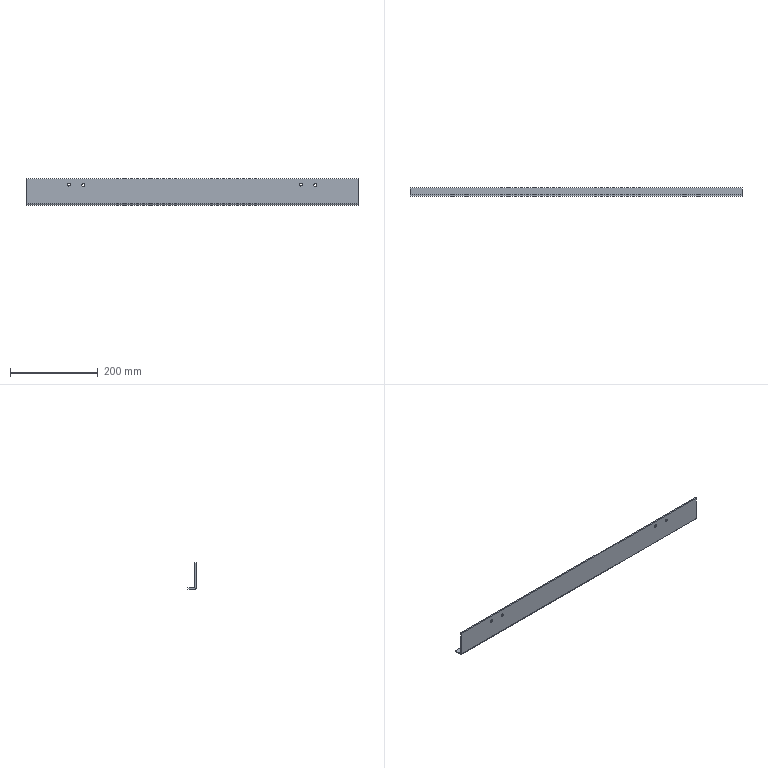Part | STEP file | HESS-408-70-15W-W-46-outer case reinforcing rib 5 | 1 solid | 18 faces | box 755 x 18.5 x 60 mm | volume 169016 mm3 | cylinder 10 | plane 8 | commonest cylinder face diameters 6.8 x8 0.2 x1 6.2 x1
STEP:
#1=CARTESIAN_POINT('',(0.,0.,0.));
#2=DIRECTION('',(0.,0.,1.));
#3=DIRECTION('',(1.,0.,0.));
#4=AXIS2_PLACEMENT_3D('',#1,#2,#3);
#5=CARTESIAN_POINT('',(-247.,0.,12.1));
#6=VERTEX_POINT('',#5);
#7=CARTESIAN_POINT('',(-247.,-3.,12.1));
#8=VERTEX_POINT('',#7);
#9=CARTESIAN_POINT('',(-247.,7.,12.1));
#10=DIRECTION('',(0.,-1.,0.));
#11=VECTOR('',#10,1.);
#12=LINE('',#9,#11);
#13=CARTESIAN_POINT('',(-247.,7.,15.5));
#14=DIRECTION('',(0.,-1.,0.));
#15=DIRECTION('',(0.,0.,-1.));
#16=AXIS2_PLACEMENT_3D('',#13,#14,#15);
#17=CYLINDRICAL_SURFACE('',#16,3.4);
#18=CARTESIAN_POINT('',(6.283,0.));
#19=DIRECTION('',(0.,1.));
#20=VECTOR('',#19,1.);
#21=LINE('',#18,#20);
#22=(GEOMETRIC_REPRESENTATION_CONTEXT(2)PARAMETRIC_REPRESENTATION_CONTEXT()REPRESENTATION_CONTEXT('',''));
#23=DEFINITIONAL_REPRESENTATION('',(#21),#22);
#24=PCURVE('',#17,#23);
#25=CARTESIAN_POINT('',(-247.,7.,15.5));
#26=DIRECTION('',(0.,-1.,0.));
#27=DIRECTION('',(0.,0.,-1.));
#28=AXIS2_PLACEMENT_3D('',#25,#26,#27);
#29=CYLINDRICAL_SURFACE('',#28,3.4);
#30=CARTESIAN_POINT('',(0.,0.));
#31=DIRECTION('',(0.,1.));
#32=VECTOR('',#31,1.);
#33=LINE('',#30,#32);
#34=(GEOMETRIC_REPRESENTATION_CONTEXT(2)PARAMETRIC_REPRESENTATION_CONTEXT()REPRESENTATION_CONTEXT('',''));
#35=DEFINITIONAL_REPRESENTATION('',(#33),#34);
#36=PCURVE('',#29,#35);
#37=SURFACE_CURVE('',#12,(#24,#36),.PCURVE_S1.);
#38=EDGE_CURVE('',#6,#8,#37,.T.);
#39=ORIENTED_EDGE('',*,*,#38,.T.);
#40=CARTESIAN_POINT('',(-247.,-3.,18.9));
#41=VERTEX_POINT('',#40);
#42=CARTESIAN_POINT('',(-247.,-3.,15.5));
#43=DIRECTION('',(0.,1.,0.));
#44=DIRECTION('',(0.,0.,-1.));
#45=AXIS2_PLACEMENT_3D('',#42,#43,#44);
#46=CIRCLE('',#45,3.4);
#47=CARTESIAN_POINT('',(6.283,10.));
#48=DIRECTION('',(-1.,0.));
#49=VECTOR('',#48,1.);
#50=LINE('',#47,#49);
#51=(GEOMETRIC_REPRESENTATION_CONTEXT(2)PARAMETRIC_REPRESENTATION_CONTEXT()REPRESENTATION_CONTEXT('',''));
#52=DEFINITIONAL_REPRESENTATION('',(#50),#51);
#53=PCURVE('',#17,#52);
#54=CARTESIAN_POINT('',(0.,-3.,0.));
#55=DIRECTION('',(0.,-1.,0.));
#56=DIRECTION('',(0.,0.,-1.));
#57=AXIS2_PLACEMENT_3D('',#54,#55,#56);
#58=PLANE('',#57);
#59=CARTESIAN_POINT('',(-12.1,-247.));
#60=CARTESIAN_POINT('',(-12.1,-252.889));
#61=CARTESIAN_POINT('',(-17.2,-249.944));
#62=CARTESIAN_POINT('',(-22.3,-247.));
#63=CARTESIAN_POINT('',(-17.2,-244.056));
#64=CARTESIAN_POINT('',(-12.1,-241.111));
#65=CARTESIAN_POINT('',(-12.1,-247.));
#66=(BOUNDED_CURVE()B_SPLINE_CURVE(2,(#59,#60,#61,#62,#63,#64,#65),.UNSPECIFIED.,.T.,.F.)B_SPLINE_CURVE_WITH_KNOTS((1,2,2,2,2,1),(-2.094,0.,2.094,4.189,6.283,8.378),.UNSPECIFIED.)CURVE()GEOMETRIC_REPRESENTATION_ITEM()RATIONAL_B_SPLINE_CURVE((1.,0.5,1.,0.5,1.,0.5,1.))REPRESENTATION_ITEM(''));
#67=(GEOMETRIC_REPRESENTATION_CONTEXT(2)PARAMETRIC_REPRESENTATION_CONTEXT()REPRESENTATION_CONTEXT('',''));
#68=DEFINITIONAL_REPRESENTATION('',(#66),#67);
#69=PCURVE('',#58,#68);
#70=SURFACE_CURVE('',#46,(#53,#69),.PCURVE_S1.);
#71=EDGE_CURVE('',#8,#41,#70,.T.);
#72=ORIENTED_EDGE('',*,*,#71,.T.);
#73=CARTESIAN_POINT('',(-247.,0.,18.9));
#74=VERTEX_POINT('',#73);
#75=CARTESIAN_POINT('',(-247.,7.,18.9));
#76=DIRECTION('',(0.,-1.,0.));
#77=VECTOR('',#76,1.);
#78=LINE('',#75,#77);
#79=CARTESIAN_POINT('',(3.142,0.));
#80=DIRECTION('',(0.,1.));
#81=VECTOR('',#80,1.);
#82=LINE('',#79,#81);
#83=(GEOMETRIC_REPRESENTATION_CONTEXT(2)PARAMETRIC_REPRESENTATION_CONTEXT()REPRESENTATION_CONTEXT('',''));
#84=DEFINITIONAL_REPRESENTATION('',(#82),#83);
#85=PCURVE('',#17,#84);
#86=CARTESIAN_POINT('',(3.142,0.));
#87=DIRECTION('',(0.,1.));
#88=VECTOR('',#87,1.);
#89=LINE('',#86,#88);
#90=(GEOMETRIC_REPRESENTATION_CONTEXT(2)PARAMETRIC_REPRESENTATION_CONTEXT()REPRESENTATION_CONTEXT('',''));
#91=DEFINITIONAL_REPRESENTATION('',(#89),#90);
#92=PCURVE('',#29,#91);
#93=SURFACE_CURVE('',#78,(#85,#92),.PCURVE_S1.);
#94=EDGE_CURVE('',#74,#41,#93,.T.);
#95=ORIENTED_EDGE('',*,*,#94,.F.);
#96=CARTESIAN_POINT('',(-247.,0.,15.5));
#97=DIRECTION('',(0.,-1.,0.));
#98=DIRECTION('',(0.,0.,-1.));
#99=AXIS2_PLACEMENT_3D('',#96,#97,#98);
#100=CIRCLE('',#99,3.4);
#101=CARTESIAN_POINT('',(0.,7.));
#102=DIRECTION('',(1.,0.));
#103=VECTOR('',#102,1.);
#104=LINE('',#101,#103);
#105=(GEOMETRIC_REPRESENTATION_CONTEXT(2)PARAMETRIC_REPRESENTATION_CONTEXT()REPRESENTATION_CONTEXT('',''));
#106=DEFINITIONAL_REPRESENTATION('',(#104),#105);
#107=PCURVE('',#17,#106);
#108=CARTESIAN_POINT('',(0.,0.,0.));
#109=DIRECTION('',(0.,-1.,0.));
#110=DIRECTION('',(0.,0.,-1.));
#111=AXIS2_PLACEMENT_3D('',#108,#109,#110);
#112=PLANE('',#111);
#113=CARTESIAN_POINT('',(-15.5,-247.));
#114=DIRECTION('',(1.,0.));
#115=AXIS2_PLACEMENT_2D('',#113,#114);
#116=CIRCLE('',#115,3.4);
#117=(GEOMETRIC_REPRESENTATION_CONTEXT(2)PARAMETRIC_REPRESENTATION_CONTEXT()REPRESENTATION_CONTEXT('',''));
#118=DEFINITIONAL_REPRESENTATION('',(#116),#117);
#119=PCURVE('',#112,#118);
#120=SURFACE_CURVE('',#100,(#107,#119),.PCURVE_S1.);
#121=EDGE_CURVE('',#74,#6,#120,.T.);
#122=ORIENTED_EDGE('',*,*,#121,.T.);
#123=EDGE_LOOP('',(#39,#72,#95,#122));
#124=FACE_BOUND('',#123,.F.);
#125=ADVANCED_FACE('',(#124),#17,.F.);
#126=CARTESIAN_POINT('',(280.5,0.,12.1));
#127=VERTEX_POINT('',#126);
#128=CARTESIAN_POINT('',(280.5,-3.,12.1));
#129=VERTEX_POINT('',#128);
#130=CARTESIAN_POINT('',(280.5,7.,12.1));
#131=DIRECTION('',(0.,-1.,0.));
#132=VECTOR('',#131,1.);
#133=LINE('',#130,#132);
#134=CARTESIAN_POINT('',(280.5,7.,15.5));
#135=DIRECTION('',(0.,-1.,0.));
#136=DIRECTION('',(0.,0.,-1.));
#137=AXIS2_PLACEMENT_3D('',#134,#135,#136);
#138=CYLINDRICAL_SURFACE('',#137,3.4);
#139=CARTESIAN_POINT('',(6.283,0.));
#140=DIRECTION('',(0.,1.));
#141=VECTOR('',#140,1.);
#142=LINE('',#139,#141);
#143=(GEOMETRIC_REPRESENTATION_CONTEXT(2)PARAMETRIC_REPRESENTATION_CONTEXT()REPRESENTATION_CONTEXT('',''));
#144=DEFINITIONAL_REPRESENTATION('',(#142),#143);
#145=PCURVE('',#138,#144);
#146=CARTESIAN_POINT('',(280.5,7.,15.5));
#147=DIRECTION('',(0.,-1.,0.));
#148=DIRECTION('',(0.,0.,-1.));
#149=AXIS2_PLACEMENT_3D('',#146,#147,#148);
#150=CYLINDRICAL_SURFACE('',#149,3.4);
#151=CARTESIAN_POINT('',(0.,0.));
#152=DIRECTION('',(0.,1.));
#153=VECTOR('',#152,1.);
#154=LINE('',#151,#153);
#155=(GEOMETRIC_REPRESENTATION_CONTEXT(2)PARAMETRIC_REPRESENTATION_CONTEXT()REPRESENTATION_CONTEXT('',''));
#156=DEFINITIONAL_REPRESENTATION('',(#154),#155);
#157=PCURVE('',#150,#156);
#158=SURFACE_CURVE('',#133,(#145,#157),.PCURVE_S1.);
#159=EDGE_CURVE('',#127,#129,#158,.T.);
#160=ORIENTED_EDGE('',*,*,#159,.T.);
#161=CARTESIAN_POINT('',(280.5,-3.,18.9));
#162=VERTEX_POINT('',#161);
#163=CARTESIAN_POINT('',(280.5,-3.,15.5));
#164=DIRECTION('',(0.,1.,0.));
#165=DIRECTION('',(0.,0.,-1.));
#166=AXIS2_PLACEMENT_3D('',#163,#164,#165);
#167=CIRCLE('',#166,3.4);
#168=CARTESIAN_POINT('',(6.283,10.));
#169=DIRECTION('',(-1.,0.));
#170=VECTOR('',#169,1.);
#171=LINE('',#168,#170);
#172=(GEOMETRIC_REPRESENTATION_CONTEXT(2)PARAMETRIC_REPRESENTATION_CONTEXT()REPRESENTATION_CONTEXT('',''));
#173=DEFINITIONAL_REPRESENTATION('',(#171),#172);
#174=PCURVE('',#138,#173);
#175=CARTESIAN_POINT('',(-12.1,280.5));
#176=CARTESIAN_POINT('',(-12.1,274.611));
#177=CARTESIAN_POINT('',(-17.2,277.556));
#178=CARTESIAN_POINT('',(-22.3,280.5));
#179=CARTESIAN_POINT('',(-17.2,283.444));
#180=CARTESIAN_POINT('',(-12.1,286.389));
#181=CARTESIAN_POINT('',(-12.1,280.5));
#182=(BOUNDED_CURVE()B_SPLINE_CURVE(2,(#175,#176,#177,#178,#179,#180,#181),.UNSPECIFIED.,.T.,.F.)B_SPLINE_CURVE_WITH_KNOTS((1,2,2,2,2,1),(-2.094,0.,2.094,4.189,6.283,8.378),.UNSPECIFIED.)CURVE()GEOMETRIC_REPRESENTATION_ITEM()RATIONAL_B_SPLINE_CURVE((1.,0.5,1.,0.5,1.,0.5,1.))REPRESENTATION_ITEM(''));
#183=(GEOMETRIC_REPRESENTATION_CONTEXT(2)PARAMETRIC_REPRESENTATION_CONTEXT()REPRESENTATION_CONTEXT('',''));
#184=DEFINITIONAL_REPRESENTATION('',(#182),#183);
#185=PCURVE('',#58,#184);
#186=SURFACE_CURVE('',#167,(#174,#185),.PCURVE_S1.);
#187=EDGE_CURVE('',#129,#162,#186,.T.);
#188=ORIENTED_EDGE('',*,*,#187,.T.);
#189=CARTESIAN_POINT('',(280.5,0.,18.9));
#190=VERTEX_POINT('',#189);
#191=CARTESIAN_POINT('',(280.5,7.,18.9));
#192=DIRECTION('',(0.,-1.,0.));
#193=VECTOR('',#192,1.);
#194=LINE('',#191,#193);
#195=CARTESIAN_POINT('',(3.142,0.));
#196=DIRECTION('',(0.,1.));
#197=VECTOR('',#196,1.);
#198=LINE('',#195,#197);
#199=(GEOMETRIC_REPRESENTATION_CONTEXT(2)PARAMETRIC_REPRESENTATION_CONTEXT()REPRESENTATION_CONTEXT('',''));
#200=DEFINITIONAL_REPRESENTATION('',(#198),#199);
#201=PCURVE('',#138,#200);
#202=CARTESIAN_POINT('',(3.142,0.));
#203=DIRECTION('',(0.,1.));
#204=VECTOR('',#203,1.);
#205=LINE('',#202,#204);
#206=(GEOMETRIC_REPRESENTATION_CONTEXT(2)PARAMETRIC_REPRESENTATION_CONTEXT()REPRESENTATION_CONTEXT('',''));
#207=DEFINITIONAL_REPRESENTATION('',(#205),#206);
#208=PCURVE('',#150,#207);
#209=SURFACE_CURVE('',#194,(#201,#208),.PCURVE_S1.);
#210=EDGE_CURVE('',#190,#162,#209,.T.);
#211=ORIENTED_EDGE('',*,*,#210,.F.);
#212=CARTESIAN_POINT('',(280.5,0.,15.5));
#213=DIRECTION('',(0.,-1.,0.));
#214=DIRECTION('',(0.,0.,-1.));
#215=AXIS2_PLACEMENT_3D('',#212,#213,#214);
#216=CIRCLE('',#215,3.4);
#217=CARTESIAN_POINT('',(0.,7.));
#218=DIRECTION('',(1.,0.));
#219=VECTOR('',#218,1.);
#220=LINE('',#217,#219);
#221=(GEOMETRIC_REPRESENTATION_CONTEXT(2)PARAMETRIC_REPRESENTATION_CONTEXT()REPRESENTATION_CONTEXT('',''));
#222=DEFINITIONAL_REPRESENTATION('',(#220),#221);
#223=PCURVE('',#138,#222);
#224=CARTESIAN_POINT('',(-15.5,280.5));
#225=DIRECTION('',(1.,0.));
#226=AXIS2_PLACEMENT_2D('',#224,#225);
#227=CIRCLE('',#226,3.4);
#228=(GEOMETRIC_REPRESENTATION_CONTEXT(2)PARAMETRIC_REPRESENTATION_CONTEXT()REPRESENTATION_CONTEXT('',''));
#229=DEFINITIONAL_REPRESENTATION('',(#227),#228);
#230=PCURVE('',#112,#229);
#231=SURFACE_CURVE('',#216,(#223,#230),.PCURVE_S1.);
#232=EDGE_CURVE('',#190,#127,#231,.T.);
#233=ORIENTED_EDGE('',*,*,#232,.T.);
#234=EDGE_LOOP('',(#160,#188,#211,#233));
#235=FACE_BOUND('',#234,.F.);
#236=ADVANCED_FACE('',(#235),#138,.F.);
#237=CARTESIAN_POINT('',(247.,0.,13.6));
#238=VERTEX_POINT('',#237);
#239=CARTESIAN_POINT('',(247.,-3.,13.6));
#240=VERTEX_POINT('',#239);
#241=CARTESIAN_POINT('',(247.,7.,13.6));
#242=DIRECTION('',(0.,-1.,0.));
#243=VECTOR('',#242,1.);
#244=LINE('',#241,#243);
#245=CARTESIAN_POINT('',(247.,7.,17.));
#246=DIRECTION('',(0.,-1.,0.));
#247=DIRECTION('',(0.,0.,-1.));
#248=AXIS2_PLACEMENT_3D('',#245,#246,#247);
#249=CYLINDRICAL_SURFACE('',#248,3.4);
#250=CARTESIAN_POINT('',(6.283,0.));
#251=DIRECTION('',(0.,1.));
#252=VECTOR('',#251,1.);
#253=LINE('',#250,#252);
#254=(GEOMETRIC_REPRESENTATION_CONTEXT(2)PARAMETRIC_REPRESENTATION_CONTEXT()REPRESENTATION_CONTEXT('',''));
#255=DEFINITIONAL_REPRESENTATION('',(#253),#254);
#256=PCURVE('',#249,#255);
#257=CARTESIAN_POINT('',(247.,7.,17.));
#258=DIRECTION('',(0.,-1.,0.));
#259=DIRECTION('',(0.,0.,-1.));
#260=AXIS2_PLACEMENT_3D('',#257,#258,#259);
#261=CYLINDRICAL_SURFACE('',#260,3.4);
#262=CARTESIAN_POINT('',(0.,0.));
#263=DIRECTION('',(0.,1.));
#264=VECTOR('',#263,1.);
#265=LINE('',#262,#264);
#266=(GEOMETRIC_REPRESENTATION_CONTEXT(2)PARAMETRIC_REPRESENTATION_CONTEXT()REPRESENTATION_CONTEXT('',''));
#267=DEFINITIONAL_REPRESENTATION('',(#265),#266);
#268=PCURVE('',#261,#267);
#269=SURFACE_CURVE('',#244,(#256,#268),.PCURVE_S1.);
#270=EDGE_CURVE('',#238,#240,#269,.T.);
#271=ORIENTED_EDGE('',*,*,#270,.T.);
#272=CARTESIAN_POINT('',(247.,-3.,20.4));
#273=VERTEX_POINT('',#272);
#274=CARTESIAN_POINT('',(247.,-3.,17.));
#275=DIRECTION('',(0.,1.,0.));
#276=DIRECTION('',(0.,0.,-1.));
#277=AXIS2_PLACEMENT_3D('',#274,#275,#276);
#278=CIRCLE('',#277,3.4);
#279=CARTESIAN_POINT('',(6.283,10.));
#280=DIRECTION('',(-1.,0.));
#281=VECTOR('',#280,1.);
#282=LINE('',#279,#281);
#283=(GEOMETRIC_REPRESENTATION_CONTEXT(2)PARAMETRIC_REPRESENTATION_CONTEXT()REPRESENTATION_CONTEXT('',''));
#284=DEFINITIONAL_REPRESENTATION('',(#282),#283);
#285=PCURVE('',#249,#284);
#286=CARTESIAN_POINT('',(-13.6,247.));
#287=CARTESIAN_POINT('',(-13.6,241.111));
#288=CARTESIAN_POINT('',(-18.7,244.056));
#289=CARTESIAN_POINT('',(-23.8,247.));
#290=CARTESIAN_POINT('',(-18.7,249.944));
#291=CARTESIAN_POINT('',(-13.6,252.889));
#292=CARTESIAN_POINT('',(-13.6,247.));
#293=(BOUNDED_CURVE()B_SPLINE_CURVE(2,(#286,#287,#288,#289,#290,#291,#292),.UNSPECIFIED.,.T.,.F.)B_SPLINE_CURVE_WITH_KNOTS((1,2,2,2,2,1),(-2.094,0.,2.094,4.189,6.283,8.378),.UNSPECIFIED.)CURVE()GEOMETRIC_REPRESENTATION_ITEM()RATIONAL_B_SPLINE_CURVE((1.,0.5,1.,0.5,1.,0.5,1.))REPRESENTATION_ITEM(''));
#294=(GEOMETRIC_REPRESENTATION_CONTEXT(2)PARAMETRIC_REPRESENTATION_CONTEXT()REPRESENTATION_CONTEXT('',''));
#295=DEFINITIONAL_REPRESENTATION('',(#293),#294);
#296=PCURVE('',#58,#295);
#297=SURFACE_CURVE('',#278,(#285,#296),.PCURVE_S1.);
#298=EDGE_CURVE('',#240,#273,#297,.T.);
#299=ORIENTED_EDGE('',*,*,#298,.T.);
#300=CARTESIAN_POINT('',(247.,0.,20.4));
#301=VERTEX_POINT('',#300);
#302=CARTESIAN_POINT('',(247.,7.,20.4));
#303=DIRECTION('',(0.,-1.,0.));
#304=VECTOR('',#303,1.);
#305=LINE('',#302,#304);
#306=CARTESIAN_POINT('',(3.142,0.));
#307=DIRECTION('',(0.,1.));
#308=VECTOR('',#307,1.);
#309=LINE('',#306,#308);
#310=(GEOMETRIC_REPRESENTATION_CONTEXT(2)PARAMETRIC_REPRESENTATION_CONTEXT()REPRESENTATION_CONTEXT('',''));
#311=DEFINITIONAL_REPRESENTATION('',(#309),#310);
#312=PCURVE('',#249,#311);
#313=CARTESIAN_POINT('',(3.142,0.));
#314=DIRECTION('',(0.,1.));
#315=VECTOR('',#314,1.);
#316=LINE('',#313,#315);
#317=(GEOMETRIC_REPRESENTATION_CONTEXT(2)PARAMETRIC_REPRESENTATION_CONTEXT()REPRESENTATION_CONTEXT('',''));
#318=DEFINITIONAL_REPRESENTATION('',(#316),#317);
#319=PCURVE('',#261,#318);
#320=SURFACE_CURVE('',#305,(#312,#319),.PCURVE_S1.);
#321=EDGE_CURVE('',#301,#273,#320,.T.);
#322=ORIENTED_EDGE('',*,*,#321,.F.);
#323=CARTESIAN_POINT('',(247.,0.,17.));
#324=DIRECTION('',(0.,-1.,0.));
#325=DIRECTION('',(0.,0.,-1.));
#326=AXIS2_PLACEMENT_3D('',#323,#324,#325);
#327=CIRCLE('',#326,3.4);
#328=CARTESIAN_POINT('',(0.,7.));
#329=DIRECTION('',(1.,0.));
#330=VECTOR('',#329,1.);
#331=LINE('',#328,#330);
#332=(GEOMETRIC_REPRESENTATION_CONTEXT(2)PARAMETRIC_REPRESENTATION_CONTEXT()REPRESENTATION_CONTEXT('',''));
#333=DEFINITIONAL_REPRESENTATION('',(#331),#332);
#334=PCURVE('',#249,#333);
#335=CARTESIAN_POINT('',(-17.,247.));
#336=DIRECTION('',(1.,0.));
#337=AXIS2_PLACEMENT_2D('',#335,#336);
#338=CIRCLE('',#337,3.4);
#339=(GEOMETRIC_REPRESENTATION_CONTEXT(2)PARAMETRIC_REPRESENTATION_CONTEXT()REPRESENTATION_CONTEXT('',''));
#340=DEFINITIONAL_REPRESENTATION('',(#338),#339);
#341=PCURVE('',#112,#340);
#342=SURFACE_CURVE('',#327,(#334,#341),.PCURVE_S1.);
#343=EDGE_CURVE('',#301,#238,#342,.T.);
#344=ORIENTED_EDGE('',*,*,#343,.T.);
#345=EDGE_LOOP('',(#271,#299,#322,#344));
#346=FACE_BOUND('',#345,.F.);
#347=ADVANCED_FACE('',(#346),#249,.F.);
#348=CARTESIAN_POINT('',(-280.5,0.,13.6));
#349=VERTEX_POINT('',#348);
#350=CARTESIAN_POINT('',(-280.5,-3.,13.6));
#351=VERTEX_POINT('',#350);
#352=CARTESIAN_POINT('',(-280.5,7.,13.6));
#353=DIRECTION('',(0.,-1.,0.));
#354=VECTOR('',#353,1.);
#355=LINE('',#352,#354);
#356=CARTESIAN_POINT('',(-280.5,7.,17.));
#357=DIRECTION('',(0.,-1.,0.));
#358=DIRECTION('',(0.,0.,-1.));
#359=AXIS2_PLACEMENT_3D('',#356,#357,#358);
#360=CYLINDRICAL_SURFACE('',#359,3.4);
#361=CARTESIAN_POINT('',(6.283,0.));
#362=DIRECTION('',(0.,1.));
#363=VECTOR('',#362,1.);
#364=LINE('',#361,#363);
#365=(GEOMETRIC_REPRESENTATION_CONTEXT(2)PARAMETRIC_REPRESENTATION_CONTEXT()REPRESENTATION_CONTEXT('',''));
#366=DEFINITIONAL_REPRESENTATION('',(#364),#365);
#367=PCURVE('',#360,#366);
#368=CARTESIAN_POINT('',(-280.5,7.,17.));
#369=DIRECTION('',(0.,-1.,0.));
#370=DIRECTION('',(0.,0.,-1.));
#371=AXIS2_PLACEMENT_3D('',#368,#369,#370);
#372=CYLINDRICAL_SURFACE('',#371,3.4);
#373=CARTESIAN_POINT('',(0.,0.));
#374=DIRECTION('',(0.,1.));
#375=VECTOR('',#374,1.);
#376=LINE('',#373,#375);
#377=(GEOMETRIC_REPRESENTATION_CONTEXT(2)PARAMETRIC_REPRESENTATION_CONTEXT()REPRESENTATION_CONTEXT('',''));
#378=DEFINITIONAL_REPRESENTATION('',(#376),#377);
#379=PCURVE('',#372,#378);
#380=SURFACE_CURVE('',#355,(#367,#379),.PCURVE_S1.);
#381=EDGE_CURVE('',#349,#351,#380,.T.);
#382=ORIENTED_EDGE('',*,*,#381,.T.);
#383=CARTESIAN_POINT('',(-280.5,-3.,20.4));
#384=VERTEX_POINT('',#383);
#385=CARTESIAN_POINT('',(-280.5,-3.,17.));
#386=DIRECTION('',(0.,1.,0.));
#387=DIRECTION('',(0.,0.,-1.));
#388=AXIS2_PLACEMENT_3D('',#385,#386,#387);
#389=CIRCLE('',#388,3.4);
#390=CARTESIAN_POINT('',(6.283,10.));
#391=DIRECTION('',(-1.,0.));
#392=VECTOR('',#391,1.);
#393=LINE('',#390,#392);
#394=(GEOMETRIC_REPRESENTATION_CONTEXT(2)PARAMETRIC_REPRESENTATION_CONTEXT()REPRESENTATION_CONTEXT('',''));
#395=DEFINITIONAL_REPRESENTATION('',(#393),#394);
#396=PCURVE('',#360,#395);
#397=CARTESIAN_POINT('',(-13.6,-280.5));
#398=CARTESIAN_POINT('',(-13.6,-286.389));
#399=CARTESIAN_POINT('',(-18.7,-283.444));
#400=CARTESIAN_POINT('',(-23.8,-280.5));
#401=CARTESIAN_POINT('',(-18.7,-277.556));
#402=CARTESIAN_POINT('',(-13.6,-274.611));
#403=CARTESIAN_POINT('',(-13.6,-280.5));
#404=(BOUNDED_CURVE()B_SPLINE_CURVE(2,(#397,#398,#399,#400,#401,#402,#403),.UNSPECIFIED.,.T.,.F.)B_SPLINE_CURVE_WITH_KNOTS((1,2,2,2,2,1),(-2.094,0.,2.094,4.189,6.283,8.378),.UNSPECIFIED.)CURVE()GEOMETRIC_REPRESENTATION_ITEM()RATIONAL_B_SPLINE_CURVE((1.,0.5,1.,0.5,1.,0.5,1.))REPRESENTATION_ITEM(''));
#405=(GEOMETRIC_REPRESENTATION_CONTEXT(2)PARAMETRIC_REPRESENTATION_CONTEXT()REPRESENTATION_CONTEXT('',''));
#406=DEFINITIONAL_REPRESENTATION('',(#404),#405);
#407=PCURVE('',#58,#406);
#408=SURFACE_CURVE('',#389,(#396,#407),.PCURVE_S1.);
#409=EDGE_CURVE('',#351,#384,#408,.T.);
#410=ORIENTED_EDGE('',*,*,#409,.T.);
#411=CARTESIAN_POINT('',(-280.5,0.,20.4));
#412=VERTEX_POINT('',#411);
#413=CARTESIAN_POINT('',(-280.5,7.,20.4));
#414=DIRECTION('',(0.,-1.,0.));
#415=VECTOR('',#414,1.);
#416=LINE('',#413,#415);
#417=CARTESIAN_POINT('',(3.142,0.));
#418=DIRECTION('',(0.,1.));
#419=VECTOR('',#418,1.);
#420=LINE('',#417,#419);
#421=(GEOMETRIC_REPRESENTATION_CONTEXT(2)PARAMETRIC_REPRESENTATION_CONTEXT()REPRESENTATION_CONTEXT('',''));
#422=DEFINITIONAL_REPRESENTATION('',(#420),#421);
#423=PCURVE('',#360,#422);
#424=CARTESIAN_POINT('',(3.142,0.));
#425=DIRECTION('',(0.,1.));
#426=VECTOR('',#425,1.);
#427=LINE('',#424,#426);
#428=(GEOMETRIC_REPRESENTATION_CONTEXT(2)PARAMETRIC_REPRESENTATION_CONTEXT()REPRESENTATION_CONTEXT('',''));
#429=DEFINITIONAL_REPRESENTATION('',(#427),#428);
#430=PCURVE('',#372,#429);
#431=SURFACE_CURVE('',#416,(#423,#430),.PCURVE_S1.);
#432=EDGE_CURVE('',#412,#384,#431,.T.);
#433=ORIENTED_EDGE('',*,*,#432,.F.);
#434=CARTESIAN_POINT('',(-280.5,0.,17.));
#435=DIRECTION('',(0.,-1.,0.));
#436=DIRECTION('',(0.,0.,-1.));
#437=AXIS2_PLACEMENT_3D('',#434,#435,#436);
#438=CIRCLE('',#437,3.4);
#439=CARTESIAN_POINT('',(0.,7.));
#440=DIRECTION('',(1.,0.));
#441=VECTOR('',#440,1.);
#442=LINE('',#439,#441);
#443=(GEOMETRIC_REPRESENTATION_CONTEXT(2)PARAMETRIC_REPRESENTATION_CONTEXT()REPRESENTATION_CONTEXT('',''));
#444=DEFINITIONAL_REPRESENTATION('',(#442),#443);
#445=PCURVE('',#360,#444);
#446=CARTESIAN_POINT('',(-17.,-280.5));
#447=DIRECTION('',(1.,0.));
#448=AXIS2_PLACEMENT_2D('',#446,#447);
#449=CIRCLE('',#448,3.4);
#450=(GEOMETRIC_REPRESENTATION_CONTEXT(2)PARAMETRIC_REPRESENTATION_CONTEXT()REPRESENTATION_CONTEXT('',''));
#451=DEFINITIONAL_REPRESENTATION('',(#449),#450);
#452=PCURVE('',#112,#451);
#453=SURFACE_CURVE('',#438,(#445,#452),.PCURVE_S1.);
#454=EDGE_CURVE('',#412,#349,#453,.T.);
#455=ORIENTED_EDGE('',*,*,#454,.T.);
#456=EDGE_LOOP('',(#382,#410,#433,#455));
#457=FACE_BOUND('',#456,.F.);
#458=ADVANCED_FACE('',(#457),#360,.F.);
#459=CARTESIAN_POINT('',(377.5,-3.,-26.9));
#460=VERTEX_POINT('',#459);
#461=CARTESIAN_POINT('',(377.5,-3.,30.));
#462=VERTEX_POINT('',#461);
#463=CARTESIAN_POINT('',(377.5,-3.,0.));
#464=DIRECTION('',(0.,0.,1.));
#465=VECTOR('',#464,1.);
#466=LINE('',#463,#465);
#467=CARTESIAN_POINT('',(0.,377.5));
#468=DIRECTION('',(-1.,0.));
#469=VECTOR('',#468,1.);
#470=LINE('',#467,#469);
#471=(GEOMETRIC_REPRESENTATION_CONTEXT(2)PARAMETRIC_REPRESENTATION_CONTEXT()REPRESENTATION_CONTEXT('',''));
#472=DEFINITIONAL_REPRESENTATION('',(#470),#471);
#473=PCURVE('',#58,#472);
#474=CARTESIAN_POINT('',(377.5,-3.,30.));
#475=DIRECTION('',(1.,0.,0.));
#476=DIRECTION('',(0.,0.,-1.));
#477=AXIS2_PLACEMENT_3D('',#474,#475,#476);
#478=PLANE('',#477);
#479=CARTESIAN_POINT('',(30.,0.));
#480=DIRECTION('',(-1.,0.));
#481=VECTOR('',#480,1.);
#482=LINE('',#479,#481);
#483=(GEOMETRIC_REPRESENTATION_CONTEXT(2)PARAMETRIC_REPRESENTATION_CONTEXT()REPRESENTATION_CONTEXT('',''));
#484=DEFINITIONAL_REPRESENTATION('',(#482),#483);
#485=PCURVE('',#478,#484);
#486=SURFACE_CURVE('',#466,(#473,#485),.PCURVE_S1.);
#487=EDGE_CURVE('',#460,#462,#486,.T.);
#488=ORIENTED_EDGE('',*,*,#487,.T.);
#489=CARTESIAN_POINT('',(-377.5,-3.,30.));
#490=VERTEX_POINT('',#489);
#491=CARTESIAN_POINT('',(0.,-3.,30.));
#492=DIRECTION('',(-1.,0.,0.));
#493=VECTOR('',#492,1.);
#494=LINE('',#491,#493);
#495=CARTESIAN_POINT('',(-30.,0.));
#496=DIRECTION('',(0.,-1.));
#497=VECTOR('',#496,1.);
#498=LINE('',#495,#497);
#499=(GEOMETRIC_REPRESENTATION_CONTEXT(2)PARAMETRIC_REPRESENTATION_CONTEXT()REPRESENTATION_CONTEXT('',''));
#500=DEFINITIONAL_REPRESENTATION('',(#498),#499);
#501=PCURVE('',#58,#500);
#502=CARTESIAN_POINT('',(-377.5,-3.,30.));
#503=DIRECTION('',(0.,0.,1.));
#504=DIRECTION('',(1.,0.,0.));
#505=AXIS2_PLACEMENT_3D('',#502,#503,#504);
#506=PLANE('',#505);
#507=CARTESIAN_POINT('',(377.5,0.));
#508=DIRECTION('',(-1.,0.));
#509=VECTOR('',#508,1.);
#510=LINE('',#507,#509);
#511=(GEOMETRIC_REPRESENTATION_CONTEXT(2)PARAMETRIC_REPRESENTATION_CONTEXT()REPRESENTATION_CONTEXT('',''));
#512=DEFINITIONAL_REPRESENTATION('',(#510),#511);
#513=PCURVE('',#506,#512);
#514=SURFACE_CURVE('',#494,(#501,#513),.PCURVE_S1.);
#515=EDGE_CURVE('',#462,#490,#514,.T.);
#516=ORIENTED_EDGE('',*,*,#515,.T.);
#517=CARTESIAN_POINT('',(-377.5,-3.,-26.9));
#518=VERTEX_POINT('',#517);
#519=CARTESIAN_POINT('',(-377.5,-3.,0.));
#520=DIRECTION('',(0.,0.,-1.));
#521=VECTOR('',#520,1.);
#522=LINE('',#519,#521);
#523=CARTESIAN_POINT('',(0.,-377.5));
#524=DIRECTION('',(1.,0.));
#525=VECTOR('',#524,1.);
#526=LINE('',#523,#525);
#527=(GEOMETRIC_REPRESENTATION_CONTEXT(2)PARAMETRIC_REPRESENTATION_CONTEXT()REPRESENTATION_CONTEXT('',''));
#528=DEFINITIONAL_REPRESENTATION('',(#526),#527);
#529=PCURVE('',#58,#528);
#530=CARTESIAN_POINT('',(-377.5,-3.,30.));
#531=DIRECTION('',(-1.,0.,0.));
#532=DIRECTION('',(0.,0.,1.));
#533=AXIS2_PLACEMENT_3D('',#530,#531,#532);
#534=PLANE('',#533);
#535=CARTESIAN_POINT('',(-30.,0.));
#536=DIRECTION('',(-1.,0.));
#537=VECTOR('',#536,1.);
#538=LINE('',#535,#537);
#539=(GEOMETRIC_REPRESENTATION_CONTEXT(2)PARAMETRIC_REPRESENTATION_CONTEXT()REPRESENTATION_CONTEXT('',''));
#540=DEFINITIONAL_REPRESENTATION('',(#538),#539);
#541=PCURVE('',#534,#540);
#542=SURFACE_CURVE('',#522,(#529,#541),.PCURVE_S1.);
#543=EDGE_CURVE('',#490,#518,#542,.T.);
#544=ORIENTED_EDGE('',*,*,#543,.T.);
#545=CARTESIAN_POINT('',(0.,-3.,-26.9));
#546=DIRECTION('',(1.,0.,0.));
#547=VECTOR('',#546,1.);
#548=LINE('',#545,#547);
#549=CARTESIAN_POINT('',(26.9,0.));
#550=DIRECTION('',(0.,1.));
#551=VECTOR('',#550,1.);
#552=LINE('',#549,#551);
#553=(GEOMETRIC_REPRESENTATION_CONTEXT(2)PARAMETRIC_REPRESENTATION_CONTEXT()REPRESENTATION_CONTEXT('',''));
#554=DEFINITIONAL_REPRESENTATION('',(#552),#553);
#555=PCURVE('',#58,#554);
#556=CARTESIAN_POINT('',(-377.5,0.1,-26.9));
#557=DIRECTION('',(-1.,0.,0.));
#558=DIRECTION('',(0.,-1.,0.));
#559=AXIS2_PLACEMENT_3D('',#556,#557,#558);
#560=CYLINDRICAL_SURFACE('',#559,3.1);
#561=CARTESIAN_POINT('',(6.283,-377.5));
#562=DIRECTION('',(0.,-1.));
#563=VECTOR('',#562,1.);
#564=LINE('',#561,#563);
#565=(GEOMETRIC_REPRESENTATION_CONTEXT(2)PARAMETRIC_REPRESENTATION_CONTEXT()REPRESENTATION_CONTEXT('',''));
#566=DEFINITIONAL_REPRESENTATION('',(#564),#565);
#567=PCURVE('',#560,#566);
#568=SURFACE_CURVE('',#548,(#555,#567),.PCURVE_S1.);
#569=EDGE_CURVE('',#518,#460,#568,.T.);
#570=ORIENTED_EDGE('',*,*,#569,.T.);
#571=EDGE_LOOP('',(#488,#516,#544,#570));
#572=FACE_BOUND('',#571,.T.);
#573=ORIENTED_EDGE('',*,*,#71,.T.);
#574=CARTESIAN_POINT('',(-247.,-3.,15.5));
#575=DIRECTION('',(0.,1.,0.));
#576=DIRECTION('',(0.,0.,-1.));
#577=AXIS2_PLACEMENT_3D('',#574,#575,#576);
#578=CIRCLE('',#577,3.4);
#579=CARTESIAN_POINT('',(-12.1,-247.));
#580=CARTESIAN_POINT('',(-12.1,-252.889));
#581=CARTESIAN_POINT('',(-17.2,-249.944));
#582=CARTESIAN_POINT('',(-22.3,-247.));
#583=CARTESIAN_POINT('',(-17.2,-244.056));
#584=CARTESIAN_POINT('',(-12.1,-241.111));
#585=CARTESIAN_POINT('',(-12.1,-247.));
#586=(BOUNDED_CURVE()B_SPLINE_CURVE(2,(#579,#580,#581,#582,#583,#584,#585),.UNSPECIFIED.,.T.,.F.)B_SPLINE_CURVE_WITH_KNOTS((1,2,2,2,2,1),(-2.094,0.,2.094,4.189,6.283,8.378),.UNSPECIFIED.)CURVE()GEOMETRIC_REPRESENTATION_ITEM()RATIONAL_B_SPLINE_CURVE((1.,0.5,1.,0.5,1.,0.5,1.))REPRESENTATION_ITEM(''));
#587=(GEOMETRIC_REPRESENTATION_CONTEXT(2)PARAMETRIC_REPRESENTATION_CONTEXT()REPRESENTATION_CONTEXT('',''));
#588=DEFINITIONAL_REPRESENTATION('',(#586),#587);
#589=PCURVE('',#58,#588);
#590=CARTESIAN_POINT('',(6.283,10.));
#591=DIRECTION('',(-1.,0.));
#592=VECTOR('',#591,1.);
#593=LINE('',#590,#592);
#594=(GEOMETRIC_REPRESENTATION_CONTEXT(2)PARAMETRIC_REPRESENTATION_CONTEXT()REPRESENTATION_CONTEXT('',''));
#595=DEFINITIONAL_REPRESENTATION('',(#593),#594);
#596=PCURVE('',#29,#595);
#597=SURFACE_CURVE('',#578,(#589,#596),.PCURVE_S1.);
#598=EDGE_CURVE('',#41,#8,#597,.T.);
#599=ORIENTED_EDGE('',*,*,#598,.T.);
#600=EDGE_LOOP('',(#573,#599));
#601=FACE_BOUND('',#600,.T.);
#602=ORIENTED_EDGE('',*,*,#187,.T.);
#603=CARTESIAN_POINT('',(280.5,-3.,15.5));
#604=DIRECTION('',(0.,1.,0.));
#605=DIRECTION('',(0.,0.,-1.));
#606=AXIS2_PLACEMENT_3D('',#603,#604,#605);
#607=CIRCLE('',#606,3.4);
#608=CARTESIAN_POINT('',(-12.1,280.5));
#609=CARTESIAN_POINT('',(-12.1,274.611));
#610=CARTESIAN_POINT('',(-17.2,277.556));
#611=CARTESIAN_POINT('',(-22.3,280.5));
#612=CARTESIAN_POINT('',(-17.2,283.444));
#613=CARTESIAN_POINT('',(-12.1,286.389));
#614=CARTESIAN_POINT('',(-12.1,280.5));
#615=(BOUNDED_CURVE()B_SPLINE_CURVE(2,(#608,#609,#610,#611,#612,#613,#614),.UNSPECIFIED.,.T.,.F.)B_SPLINE_CURVE_WITH_KNOTS((1,2,2,2,2,1),(-2.094,0.,2.094,4.189,6.283,8.378),.UNSPECIFIED.)CURVE()GEOMETRIC_REPRESENTATION_ITEM()RATIONAL_B_SPLINE_CURVE((1.,0.5,1.,0.5,1.,0.5,1.))REPRESENTATION_ITEM(''));
#616=(GEOMETRIC_REPRESENTATION_CONTEXT(2)PARAMETRIC_REPRESENTATION_CONTEXT()REPRESENTATION_CONTEXT('',''));
#617=DEFINITIONAL_REPRESENTATION('',(#615),#616);
#618=PCURVE('',#58,#617);
#619=CARTESIAN_POINT('',(6.283,10.));
#620=DIRECTION('',(-1.,0.));
#621=VECTOR('',#620,1.);
#622=LINE('',#619,#621);
#623=(GEOMETRIC_REPRESENTATION_CONTEXT(2)PARAMETRIC_REPRESENTATION_CONTEXT()REPRESENTATION_CONTEXT('',''));
#624=DEFINITIONAL_REPRESENTATION('',(#622),#623);
#625=PCURVE('',#150,#624);
#626=SURFACE_CURVE('',#607,(#618,#625),.PCURVE_S1.);
#627=EDGE_CURVE('',#162,#129,#626,.T.);
#628=ORIENTED_EDGE('',*,*,#627,.T.);
#629=EDGE_LOOP('',(#602,#628));
#630=FACE_BOUND('',#629,.T.);
#631=ORIENTED_EDGE('',*,*,#298,.T.);
#632=CARTESIAN_POINT('',(247.,-3.,17.));
#633=DIRECTION('',(0.,1.,0.));
#634=DIRECTION('',(0.,0.,-1.));
#635=AXIS2_PLACEMENT_3D('',#632,#633,#634);
#636=CIRCLE('',#635,3.4);
#637=CARTESIAN_POINT('',(-13.6,247.));
#638=CARTESIAN_POINT('',(-13.6,241.111));
#639=CARTESIAN_POINT('',(-18.7,244.056));
#640=CARTESIAN_POINT('',(-23.8,247.));
#641=CARTESIAN_POINT('',(-18.7,249.944));
#642=CARTESIAN_POINT('',(-13.6,252.889));
#643=CARTESIAN_POINT('',(-13.6,247.));
#644=(BOUNDED_CURVE()B_SPLINE_CURVE(2,(#637,#638,#639,#640,#641,#642,#643),.UNSPECIFIED.,.T.,.F.)B_SPLINE_CURVE_WITH_KNOTS((1,2,2,2,2,1),(-2.094,0.,2.094,4.189,6.283,8.378),.UNSPECIFIED.)CURVE()GEOMETRIC_REPRESENTATION_ITEM()RATIONAL_B_SPLINE_CURVE((1.,0.5,1.,0.5,1.,0.5,1.))REPRESENTATION_ITEM(''));
#645=(GEOMETRIC_REPRESENTATION_CONTEXT(2)PARAMETRIC_REPRESENTATION_CONTEXT()REPRESENTATION_CONTEXT('',''));
#646=DEFINITIONAL_REPRESENTATION('',(#644),#645);
#647=PCURVE('',#58,#646);
#648=CARTESIAN_POINT('',(6.283,10.));
#649=DIRECTION('',(-1.,0.));
#650=VECTOR('',#649,1.);
#651=LINE('',#648,#650);
#652=(GEOMETRIC_REPRESENTATION_CONTEXT(2)PARAMETRIC_REPRESENTATION_CONTEXT()REPRESENTATION_CONTEXT('',''));
#653=DEFINITIONAL_REPRESENTATION('',(#651),#652);
#654=PCURVE('',#261,#653);
#655=SURFACE_CURVE('',#636,(#647,#654),.PCURVE_S1.);
#656=EDGE_CURVE('',#273,#240,#655,.T.);
#657=ORIENTED_EDGE('',*,*,#656,.T.);
#658=EDGE_LOOP('',(#631,#657));
#659=FACE_BOUND('',#658,.T.);
#660=ORIENTED_EDGE('',*,*,#409,.T.);
#661=CARTESIAN_POINT('',(-280.5,-3.,17.));
#662=DIRECTION('',(0.,1.,0.));
#663=DIRECTION('',(0.,0.,-1.));
#664=AXIS2_PLACEMENT_3D('',#661,#662,#663);
#665=CIRCLE('',#664,3.4);
#666=CARTESIAN_POINT('',(-13.6,-280.5));
#667=CARTESIAN_POINT('',(-13.6,-286.389));
#668=CARTESIAN_POINT('',(-18.7,-283.444));
#669=CARTESIAN_POINT('',(-23.8,-280.5));
#670=CARTESIAN_POINT('',(-18.7,-277.556));
#671=CARTESIAN_POINT('',(-13.6,-274.611));
#672=CARTESIAN_POINT('',(-13.6,-280.5));
#673=(BOUNDED_CURVE()B_SPLINE_CURVE(2,(#666,#667,#668,#669,#670,#671,#672),.UNSPECIFIED.,.T.,.F.)B_SPLINE_CURVE_WITH_KNOTS((1,2,2,2,2,1),(-2.094,0.,2.094,4.189,6.283,8.378),.UNSPECIFIED.)CURVE()GEOMETRIC_REPRESENTATION_ITEM()RATIONAL_B_SPLINE_CURVE((1.,0.5,1.,0.5,1.,0.5,1.))REPRESENTATION_ITEM(''));
#674=(GEOMETRIC_REPRESENTATION_CONTEXT(2)PARAMETRIC_REPRESENTATION_CONTEXT()REPRESENTATION_CONTEXT('',''));
#675=DEFINITIONAL_REPRESENTATION('',(#673),#674);
#676=PCURVE('',#58,#675);
#677=CARTESIAN_POINT('',(6.283,10.));
#678=DIRECTION('',(-1.,0.));
#679=VECTOR('',#678,1.);
#680=LINE('',#677,#679);
#681=(GEOMETRIC_REPRESENTATION_CONTEXT(2)PARAMETRIC_REPRESENTATION_CONTEXT()REPRESENTATION_CONTEXT('',''));
#682=DEFINITIONAL_REPRESENTATION('',(#680),#681);
#683=PCURVE('',#372,#682);
#684=SURFACE_CURVE('',#665,(#676,#683),.PCURVE_S1.);
#685=EDGE_CURVE('',#384,#351,#684,.T.);
#686=ORIENTED_EDGE('',*,*,#685,.T.);
#687=EDGE_LOOP('',(#660,#686));
#688=FACE_BOUND('',#687,.T.);
#689=ADVANCED_FACE('',(#572,#601,#630,#659,#688),#58,.T.);
#690=ORIENTED_EDGE('',*,*,#515,.F.);
#691=CARTESIAN_POINT('',(377.5,0.,30.));
#692=VERTEX_POINT('',#691);
#693=CARTESIAN_POINT('',(377.5,-3.,30.));
#694=DIRECTION('',(0.,1.,0.));
#695=VECTOR('',#694,1.);
#696=LINE('',#693,#695);
#697=CARTESIAN_POINT('',(755.,0.));
#698=DIRECTION('',(0.,1.));
#699=VECTOR('',#698,1.);
#700=LINE('',#697,#699);
#701=(GEOMETRIC_REPRESENTATION_CONTEXT(2)PARAMETRIC_REPRESENTATION_CONTEXT()REPRESENTATION_CONTEXT('',''));
#702=DEFINITIONAL_REPRESENTATION('',(#700),#701);
#703=PCURVE('',#506,#702);
#704=CARTESIAN_POINT('',(0.,0.));
#705=DIRECTION('',(0.,1.));
#706=VECTOR('',#705,1.);
#707=LINE('',#704,#706);
#708=(GEOMETRIC_REPRESENTATION_CONTEXT(2)PARAMETRIC_REPRESENTATION_CONTEXT()REPRESENTATION_CONTEXT('',''));
#709=DEFINITIONAL_REPRESENTATION('',(#707),#708);
#710=PCURVE('',#478,#709);
#711=SURFACE_CURVE('',#696,(#703,#710),.PCURVE_S1.);
#712=EDGE_CURVE('',#462,#692,#711,.T.);
#713=ORIENTED_EDGE('',*,*,#712,.T.);
#714=CARTESIAN_POINT('',(-377.5,0.,30.));
#715=VERTEX_POINT('',#714);
#716=CARTESIAN_POINT('',(-377.5,0.,30.));
#717=DIRECTION('',(-1.,0.,0.));
#718=VECTOR('',#717,1.);
#719=LINE('',#716,#718);
#720=CARTESIAN_POINT('',(0.,3.));
#721=DIRECTION('',(-1.,0.));
#722=VECTOR('',#721,1.);
#723=LINE('',#720,#722);
#724=(GEOMETRIC_REPRESENTATION_CONTEXT(2)PARAMETRIC_REPRESENTATION_CONTEXT()REPRESENTATION_CONTEXT('',''));
#725=DEFINITIONAL_REPRESENTATION('',(#723),#724);
#726=PCURVE('',#506,#725);
#727=CARTESIAN_POINT('',(-30.,-377.5));
#728=DIRECTION('',(0.,-1.));
#729=VECTOR('',#728,1.);
#730=LINE('',#727,#729);
#731=(GEOMETRIC_REPRESENTATION_CONTEXT(2)PARAMETRIC_REPRESENTATION_CONTEXT()REPRESENTATION_CONTEXT('',''));
#732=DEFINITIONAL_REPRESENTATION('',(#730),#731);
#733=PCURVE('',#112,#732);
#734=SURFACE_CURVE('',#719,(#726,#733),.PCURVE_S1.);
#735=EDGE_CURVE('',#692,#715,#734,.T.);
#736=ORIENTED_EDGE('',*,*,#735,.T.);
#737=CARTESIAN_POINT('',(-377.5,-3.,30.));
#738=DIRECTION('',(0.,-1.,0.));
#739=VECTOR('',#738,1.);
#740=LINE('',#737,#739);
#741=CARTESIAN_POINT('',(0.,0.));
#742=DIRECTION('',(0.,-1.));
#743=VECTOR('',#742,1.);
#744=LINE('',#741,#743);
#745=(GEOMETRIC_REPRESENTATION_CONTEXT(2)PARAMETRIC_REPRESENTATION_CONTEXT()REPRESENTATION_CONTEXT('',''));
#746=DEFINITIONAL_REPRESENTATION('',(#744),#745);
#747=PCURVE('',#506,#746);
#748=CARTESIAN_POINT('',(0.,0.));
#749=DIRECTION('',(0.,-1.));
#750=VECTOR('',#749,1.);
#751=LINE('',#748,#750);
#752=(GEOMETRIC_REPRESENTATION_CONTEXT(2)PARAMETRIC_REPRESENTATION_CONTEXT()REPRESENTATION_CONTEXT('',''));
#753=DEFINITIONAL_REPRESENTATION('',(#751),#752);
#754=PCURVE('',#534,#753);
#755=SURFACE_CURVE('',#740,(#747,#754),.PCURVE_S1.);
#756=EDGE_CURVE('',#715,#490,#755,.T.);
#757=ORIENTED_EDGE('',*,*,#756,.T.);
#758=EDGE_LOOP('',(#690,#713,#736,#757));
#759=FACE_BOUND('',#758,.T.);
#760=ADVANCED_FACE('',(#759),#506,.T.);
#761=ORIENTED_EDGE('',*,*,#712,.F.);
#762=ORIENTED_EDGE('',*,*,#487,.F.);
#763=CARTESIAN_POINT('',(377.5,0.1,-30.));
#764=VERTEX_POINT('',#763);
#765=CARTESIAN_POINT('',(377.5,0.1,-26.9));
#766=DIRECTION('',(-1.,0.,0.));
#767=DIRECTION('',(0.,-1.,0.));
#768=AXIS2_PLACEMENT_3D('',#765,#766,#767);
#769=CIRCLE('',#768,3.1);
#770=CARTESIAN_POINT('',(56.9,0.));
#771=CARTESIAN_POINT('',(51.531,0.));
#772=CARTESIAN_POINT('',(54.215,4.65));
#773=CARTESIAN_POINT('',(56.9,9.3));
#774=CARTESIAN_POINT('',(59.585,4.65));
#775=CARTESIAN_POINT('',(62.269,0.));
#776=CARTESIAN_POINT('',(56.9,0.));
#777=(BOUNDED_CURVE()B_SPLINE_CURVE(2,(#770,#771,#772,#773,#774,#775,#776),.UNSPECIFIED.,.T.,.F.)B_SPLINE_CURVE_WITH_KNOTS((1,2,2,2,2,1),(-2.094,0.,2.094,4.189,6.283,8.378),.UNSPECIFIED.)CURVE()GEOMETRIC_REPRESENTATION_ITEM()RATIONAL_B_SPLINE_CURVE((1.,0.5,1.,0.5,1.,0.5,1.))REPRESENTATION_ITEM(''));
#778=(GEOMETRIC_REPRESENTATION_CONTEXT(2)PARAMETRIC_REPRESENTATION_CONTEXT()REPRESENTATION_CONTEXT('',''));
#779=DEFINITIONAL_REPRESENTATION('',(#777),#778);
#780=PCURVE('',#478,#779);
#781=CARTESIAN_POINT('',(0.,-755.));
#782=DIRECTION('',(1.,0.));
#783=VECTOR('',#782,1.);
#784=LINE('',#781,#783);
#785=(GEOMETRIC_REPRESENTATION_CONTEXT(2)PARAMETRIC_REPRESENTATION_CONTEXT()REPRESENTATION_CONTEXT('',''));
#786=DEFINITIONAL_REPRESENTATION('',(#784),#785);
#787=PCURVE('',#560,#786);
#788=SURFACE_CURVE('',#769,(#780,#787),.PCURVE_S1.);
#789=EDGE_CURVE('',#764,#460,#788,.T.);
#790=ORIENTED_EDGE('',*,*,#789,.F.);
#791=CARTESIAN_POINT('',(377.5,15.5,-30.));
#792=VERTEX_POINT('',#791);
#793=CARTESIAN_POINT('',(377.5,0.,-30.));
#794=DIRECTION('',(0.,1.,0.));
#795=VECTOR('',#794,1.);
#796=LINE('',#793,#795);
#797=CARTESIAN_POINT('',(60.,3.));
#798=DIRECTION('',(0.,1.));
#799=VECTOR('',#798,1.);
#800=LINE('',#797,#799);
#801=(GEOMETRIC_REPRESENTATION_CONTEXT(2)PARAMETRIC_REPRESENTATION_CONTEXT()REPRESENTATION_CONTEXT('',''));
#802=DEFINITIONAL_REPRESENTATION('',(#800),#801);
#803=PCURVE('',#478,#802);
#804=CARTESIAN_POINT('',(0.,0.,-30.));
#805=DIRECTION('',(0.,0.,1.));
#806=DIRECTION('',(0.,-1.,0.));
#807=AXIS2_PLACEMENT_3D('',#804,#805,#806);
#808=PLANE('',#807);
#809=CARTESIAN_POINT('',(0.,377.5));
#810=DIRECTION('',(-1.,0.));
#811=VECTOR('',#810,1.);
#812=LINE('',#809,#811);
#813=(GEOMETRIC_REPRESENTATION_CONTEXT(2)PARAMETRIC_REPRESENTATION_CONTEXT()REPRESENTATION_CONTEXT('',''));
#814=DEFINITIONAL_REPRESENTATION('',(#812),#813);
#815=PCURVE('',#808,#814);
#816=SURFACE_CURVE('',#796,(#803,#815),.PCURVE_S1.);
#817=EDGE_CURVE('',#764,#792,#816,.T.);
#818=ORIENTED_EDGE('',*,*,#817,.T.);
#819=CARTESIAN_POINT('',(377.5,15.5,-27.));
#820=VERTEX_POINT('',#819);
#821=CARTESIAN_POINT('',(377.5,15.5,-30.));
#822=DIRECTION('',(0.,0.,-1.));
#823=VECTOR('',#822,1.);
#824=LINE('',#821,#823);
#825=CARTESIAN_POINT('',(60.,18.5));
#826=DIRECTION('',(1.,0.));
#827=VECTOR('',#826,1.);
#828=LINE('',#825,#827);
#829=(GEOMETRIC_REPRESENTATION_CONTEXT(2)PARAMETRIC_REPRESENTATION_CONTEXT()REPRESENTATION_CONTEXT('',''));
#830=DEFINITIONAL_REPRESENTATION('',(#828),#829);
#831=PCURVE('',#478,#830);
#832=CARTESIAN_POINT('',(377.5,15.5,-30.));
#833=DIRECTION('',(0.,-1.,0.));
#834=DIRECTION('',(0.,0.,-1.));
#835=AXIS2_PLACEMENT_3D('',#832,#833,#834);
#836=PLANE('',#835);
#837=CARTESIAN_POINT('',(0.,0.));
#838=DIRECTION('',(1.,0.));
#839=VECTOR('',#838,1.);
#840=LINE('',#837,#839);
#841=(GEOMETRIC_REPRESENTATION_CONTEXT(2)PARAMETRIC_REPRESENTATION_CONTEXT()REPRESENTATION_CONTEXT('',''));
#842=DEFINITIONAL_REPRESENTATION('',(#840),#841);
#843=PCURVE('',#836,#842);
#844=SURFACE_CURVE('',#824,(#831,#843),.PCURVE_S1.);
#845=EDGE_CURVE('',#820,#792,#844,.T.);
#846=ORIENTED_EDGE('',*,*,#845,.F.);
#847=CARTESIAN_POINT('',(377.5,0.1,-27.));
#848=VERTEX_POINT('',#847);
#849=CARTESIAN_POINT('',(377.5,0.,-27.));
#850=DIRECTION('',(0.,1.,0.));
#851=VECTOR('',#850,1.);
#852=LINE('',#849,#851);
#853=CARTESIAN_POINT('',(57.,3.));
#854=DIRECTION('',(0.,1.));
#855=VECTOR('',#854,1.);
#856=LINE('',#853,#855);
#857=(GEOMETRIC_REPRESENTATION_CONTEXT(2)PARAMETRIC_REPRESENTATION_CONTEXT()REPRESENTATION_CONTEXT('',''));
#858=DEFINITIONAL_REPRESENTATION('',(#856),#857);
#859=PCURVE('',#478,#858);
#860=CARTESIAN_POINT('',(0.,0.,-27.));
#861=DIRECTION('',(0.,0.,1.));
#862=DIRECTION('',(0.,-1.,0.));
#863=AXIS2_PLACEMENT_3D('',#860,#861,#862);
#864=PLANE('',#863);
#865=CARTESIAN_POINT('',(0.,377.5));
#866=DIRECTION('',(-1.,0.));
#867=VECTOR('',#866,1.);
#868=LINE('',#865,#867);
#869=(GEOMETRIC_REPRESENTATION_CONTEXT(2)PARAMETRIC_REPRESENTATION_CONTEXT()REPRESENTATION_CONTEXT('',''));
#870=DEFINITIONAL_REPRESENTATION('',(#868),#869);
#871=PCURVE('',#864,#870);
#872=SURFACE_CURVE('',#852,(#859,#871),.PCURVE_S1.);
#873=EDGE_CURVE('',#848,#820,#872,.T.);
#874=ORIENTED_EDGE('',*,*,#873,.F.);
#875=CARTESIAN_POINT('',(377.5,0.,-26.9));
#876=VERTEX_POINT('',#875);
#877=CARTESIAN_POINT('',(377.5,0.1,-26.9));
#878=DIRECTION('',(-1.,0.,0.));
#879=DIRECTION('',(0.,-1.,0.));
#880=AXIS2_PLACEMENT_3D('',#877,#878,#879);
#881=CIRCLE('',#880,0.1);
#882=CARTESIAN_POINT('',(56.9,3.));
#883=CARTESIAN_POINT('',(56.727,3.));
#884=CARTESIAN_POINT('',(56.813,3.15));
#885=CARTESIAN_POINT('',(56.9,3.3));
#886=CARTESIAN_POINT('',(56.987,3.15));
#887=CARTESIAN_POINT('',(57.073,3.));
#888=CARTESIAN_POINT('',(56.9,3.));
#889=(BOUNDED_CURVE()B_SPLINE_CURVE(2,(#882,#883,#884,#885,#886,#887,#888),.UNSPECIFIED.,.T.,.F.)B_SPLINE_CURVE_WITH_KNOTS((1,2,2,2,2,1),(-2.094,0.,2.094,4.189,6.283,8.378),.UNSPECIFIED.)CURVE()GEOMETRIC_REPRESENTATION_ITEM()RATIONAL_B_SPLINE_CURVE((1.,0.5,1.,0.5,1.,0.5,1.))REPRESENTATION_ITEM(''));
#890=(GEOMETRIC_REPRESENTATION_CONTEXT(2)PARAMETRIC_REPRESENTATION_CONTEXT()REPRESENTATION_CONTEXT('',''));
#891=DEFINITIONAL_REPRESENTATION('',(#889),#890);
#892=PCURVE('',#478,#891);
#893=CARTESIAN_POINT('',(-377.5,0.1,-26.9));
#894=DIRECTION('',(-1.,0.,0.));
#895=DIRECTION('',(0.,-1.,0.));
#896=AXIS2_PLACEMENT_3D('',#893,#894,#895);
#897=CYLINDRICAL_SURFACE('',#896,0.1);
#898=CARTESIAN_POINT('',(0.,-755.));
#899=DIRECTION('',(1.,0.));
#900=VECTOR('',#899,1.);
#901=LINE('',#898,#900);
#902=(GEOMETRIC_REPRESENTATION_CONTEXT(2)PARAMETRIC_REPRESENTATION_CONTEXT()REPRESENTATION_CONTEXT('',''));
#903=DEFINITIONAL_REPRESENTATION('',(#901),#902);
#904=PCURVE('',#897,#903);
#905=SURFACE_CURVE('',#881,(#892,#904),.PCURVE_S1.);
#906=EDGE_CURVE('',#848,#876,#905,.T.);
#907=ORIENTED_EDGE('',*,*,#906,.T.);
#908=CARTESIAN_POINT('',(377.5,0.,30.));
#909=DIRECTION('',(0.,0.,1.));
#910=VECTOR('',#909,1.);
#911=LINE('',#908,#910);
#912=CARTESIAN_POINT('',(0.,3.));
#913=DIRECTION('',(-1.,0.));
#914=VECTOR('',#913,1.);
#915=LINE('',#912,#914);
#916=(GEOMETRIC_REPRESENTATION_CONTEXT(2)PARAMETRIC_REPRESENTATION_CONTEXT()REPRESENTATION_CONTEXT('',''));
#917=DEFINITIONAL_REPRESENTATION('',(#915),#916);
#918=PCURVE('',#478,#917);
#919=CARTESIAN_POINT('',(-30.,377.5));
#920=DIRECTION('',(-1.,0.));
#921=VECTOR('',#920,1.);
#922=LINE('',#919,#921);
#923=(GEOMETRIC_REPRESENTATION_CONTEXT(2)PARAMETRIC_REPRESENTATION_CONTEXT()REPRESENTATION_CONTEXT('',''));
#924=DEFINITIONAL_REPRESENTATION('',(#922),#923);
#925=PCURVE('',#112,#924);
#926=SURFACE_CURVE('',#911,(#918,#925),.PCURVE_S1.);
#927=EDGE_CURVE('',#876,#692,#926,.T.);
#928=ORIENTED_EDGE('',*,*,#927,.T.);
#929=EDGE_LOOP('',(#761,#762,#790,#818,#846,#874,#907,#928));
#930=FACE_BOUND('',#929,.T.);
#931=ADVANCED_FACE('',(#930),#478,.T.);
#932=CARTESIAN_POINT('',(-377.5,0.1,-30.));
#933=VERTEX_POINT('',#932);
#934=CARTESIAN_POINT('',(-377.5,0.1,-30.));
#935=DIRECTION('',(1.,0.,0.));
#936=VECTOR('',#935,1.);
#937=LINE('',#934,#936);
#938=CARTESIAN_POINT('',(4.712,0.));
#939=DIRECTION('',(0.,-1.));
#940=VECTOR('',#939,1.);
#941=LINE('',#938,#940);
#942=(GEOMETRIC_REPRESENTATION_CONTEXT(2)PARAMETRIC_REPRESENTATION_CONTEXT()REPRESENTATION_CONTEXT('',''));
#943=DEFINITIONAL_REPRESENTATION('',(#941),#942);
#944=PCURVE('',#560,#943);
#945=CARTESIAN_POINT('',(-0.1,-377.5));
#946=DIRECTION('',(0.,1.));
#947=VECTOR('',#946,1.);
#948=LINE('',#945,#947);
#949=(GEOMETRIC_REPRESENTATION_CONTEXT(2)PARAMETRIC_REPRESENTATION_CONTEXT()REPRESENTATION_CONTEXT('',''));
#950=DEFINITIONAL_REPRESENTATION('',(#948),#949);
#951=PCURVE('',#808,#950);
#952=SURFACE_CURVE('',#937,(#944,#951),.PCURVE_S1.);
#953=EDGE_CURVE('',#933,#764,#952,.T.);
#954=ORIENTED_EDGE('',*,*,#953,.T.);
#955=ORIENTED_EDGE('',*,*,#789,.T.);
#956=ORIENTED_EDGE('',*,*,#569,.F.);
#957=CARTESIAN_POINT('',(-377.5,0.1,-26.9));
#958=DIRECTION('',(1.,0.,0.));
#959=DIRECTION('',(0.,-1.,0.));
#960=AXIS2_PLACEMENT_3D('',#957,#958,#959);
#961=CIRCLE('',#960,3.1);
#962=CARTESIAN_POINT('',(6.283,0.));
#963=DIRECTION('',(-1.,0.));
#964=VECTOR('',#963,1.);
#965=LINE('',#962,#964);
#966=(GEOMETRIC_REPRESENTATION_CONTEXT(2)PARAMETRIC_REPRESENTATION_CONTEXT()REPRESENTATION_CONTEXT('',''));
#967=DEFINITIONAL_REPRESENTATION('',(#965),#966);
#968=PCURVE('',#560,#967);
#969=CARTESIAN_POINT('',(-56.9,0.));
#970=CARTESIAN_POINT('',(-62.269,0.));
#971=CARTESIAN_POINT('',(-59.585,4.65));
#972=CARTESIAN_POINT('',(-56.9,9.3));
#973=CARTESIAN_POINT('',(-54.215,4.65));
#974=CARTESIAN_POINT('',(-51.531,0.));
#975=CARTESIAN_POINT('',(-56.9,0.));
#976=(BOUNDED_CURVE()B_SPLINE_CURVE(2,(#969,#970,#971,#972,#973,#974,#975),.UNSPECIFIED.,.T.,.F.)B_SPLINE_CURVE_WITH_KNOTS((1,2,2,2,2,1),(-2.094,0.,2.094,4.189,6.283,8.378),.UNSPECIFIED.)CURVE()GEOMETRIC_REPRESENTATION_ITEM()RATIONAL_B_SPLINE_CURVE((1.,0.5,1.,0.5,1.,0.5,1.))REPRESENTATION_ITEM(''));
#977=(GEOMETRIC_REPRESENTATION_CONTEXT(2)PARAMETRIC_REPRESENTATION_CONTEXT()REPRESENTATION_CONTEXT('',''));
#978=DEFINITIONAL_REPRESENTATION('',(#976),#977);
#979=PCURVE('',#534,#978);
#980=SURFACE_CURVE('',#961,(#968,#979),.PCURVE_S1.);
#981=EDGE_CURVE('',#518,#933,#980,.T.);
#982=ORIENTED_EDGE('',*,*,#981,.T.);
#983=EDGE_LOOP('',(#954,#955,#956,#982));
#984=FACE_BOUND('',#983,.T.);
#985=ADVANCED_FACE('',(#984),#560,.T.);
#986=ORIENTED_EDGE('',*,*,#543,.F.);
#987=ORIENTED_EDGE('',*,*,#756,.F.);
#988=CARTESIAN_POINT('',(-377.5,0.,-26.9));
#989=VERTEX_POINT('',#988);
#990=CARTESIAN_POINT('',(-377.5,0.,30.));
#991=DIRECTION('',(0.,0.,-1.));
#992=VECTOR('',#991,1.);
#993=LINE('',#990,#992);
#994=CARTESIAN_POINT('',(0.,3.));
#995=DIRECTION('',(-1.,0.));
#996=VECTOR('',#995,1.);
#997=LINE('',#994,#996);
#998=(GEOMETRIC_REPRESENTATION_CONTEXT(2)PARAMETRIC_REPRESENTATION_CONTEXT()REPRESENTATION_CONTEXT('',''));
#999=DEFINITIONAL_REPRESENTATION('',(#997),#998);
#1000=PCURVE('',#534,#999);
#1001=CARTESIAN_POINT('',(-30.,-377.5));
#1002=DIRECTION('',(1.,0.));
#1003=VECTOR('',#1002,1.);
#1004=LINE('',#1001,#1003);
#1005=(GEOMETRIC_REPRESENTATION_CONTEXT(2)PARAMETRIC_REPRESENTATION_CONTEXT()REPRESENTATION_CONTEXT('',''));
#1006=DEFINITIONAL_REPRESENTATION('',(#1004),#1005);
#1007=PCURVE('',#112,#1006);
#1008=SURFACE_CURVE('',#993,(#1000,#1007),.PCURVE_S1.);
#1009=EDGE_CURVE('',#715,#989,#1008,.T.);
#1010=ORIENTED_EDGE('',*,*,#1009,.T.);
#1011=CARTESIAN_POINT('',(-377.5,0.1,-27.));
#1012=VERTEX_POINT('',#1011);
#1013=CARTESIAN_POINT('',(-377.5,0.1,-26.9));
#1014=DIRECTION('',(-1.,0.,0.));
#1015=DIRECTION('',(0.,-1.,0.));
#1016=AXIS2_PLACEMENT_3D('',#1013,#1014,#1015);
#1017=CIRCLE('',#1016,0.1);
#1018=CARTESIAN_POINT('',(-56.9,3.1));
#1019=DIRECTION('',(0.,-1.));
#1020=AXIS2_PLACEMENT_2D('',#1018,#1019);
#1021=CIRCLE('',#1020,0.1);
#1022=(GEOMETRIC_REPRESENTATION_CONTEXT(2)PARAMETRIC_REPRESENTATION_CONTEXT()REPRESENTATION_CONTEXT('',''));
#1023=DEFINITIONAL_REPRESENTATION('',(#1021),#1022);
#1024=PCURVE('',#534,#1023);
#1025=CARTESIAN_POINT('',(0.,0.));
#1026=DIRECTION('',(1.,0.));
#1027=VECTOR('',#1026,1.);
#1028=LINE('',#1025,#1027);
#1029=(GEOMETRIC_REPRESENTATION_CONTEXT(2)PARAMETRIC_REPRESENTATION_CONTEXT()REPRESENTATION_CONTEXT('',''));
#1030=DEFINITIONAL_REPRESENTATION('',(#1028),#1029);
#1031=PCURVE('',#897,#1030);
#1032=SURFACE_CURVE('',#1017,(#1024,#1031),.PCURVE_S1.);
#1033=EDGE_CURVE('',#1012,#989,#1032,.T.);
#1034=ORIENTED_EDGE('',*,*,#1033,.F.);
#1035=CARTESIAN_POINT('',(-377.5,15.5,-27.));
#1036=VERTEX_POINT('',#1035);
#1037=CARTESIAN_POINT('',(-377.5,15.5,-27.));
#1038=DIRECTION('',(0.,-1.,0.));
#1039=VECTOR('',#1038,1.);
#1040=LINE('',#1037,#1039);
#1041=CARTESIAN_POINT('',(-57.,18.5));
#1042=DIRECTION('',(0.,-1.));
#1043=VECTOR('',#1042,1.);
#1044=LINE('',#1041,#1043);
#1045=(GEOMETRIC_REPRESENTATION_CONTEXT(2)PARAMETRIC_REPRESENTATION_CONTEXT()REPRESENTATION_CONTEXT('',''));
#1046=DEFINITIONAL_REPRESENTATION('',(#1044),#1045);
#1047=PCURVE('',#534,#1046);
#1048=CARTESIAN_POINT('',(-15.5,-377.5));
#1049=DIRECTION('',(1.,0.));
#1050=VECTOR('',#1049,1.);
#1051=LINE('',#1048,#1050);
#1052=(GEOMETRIC_REPRESENTATION_CONTEXT(2)PARAMETRIC_REPRESENTATION_CONTEXT()REPRESENTATION_CONTEXT('',''));
#1053=DEFINITIONAL_REPRESENTATION('',(#1051),#1052);
#1054=PCURVE('',#864,#1053);
#1055=SURFACE_CURVE('',#1040,(#1047,#1054),.PCURVE_S1.);
#1056=EDGE_CURVE('',#1036,#1012,#1055,.T.);
#1057=ORIENTED_EDGE('',*,*,#1056,.F.);
#1058=CARTESIAN_POINT('',(-377.5,15.5,-30.));
#1059=VERTEX_POINT('',#1058);
#1060=CARTESIAN_POINT('',(-377.5,15.5,-30.));
#1061=DIRECTION('',(0.,0.,1.));
#1062=VECTOR('',#1061,1.);
#1063=LINE('',#1060,#1062);
#1064=CARTESIAN_POINT('',(-60.,18.5));
#1065=DIRECTION('',(1.,0.));
#1066=VECTOR('',#1065,1.);
#1067=LINE('',#1064,#1066);
#1068=(GEOMETRIC_REPRESENTATION_CONTEXT(2)PARAMETRIC_REPRESENTATION_CONTEXT()REPRESENTATION_CONTEXT('',''));
#1069=DEFINITIONAL_REPRESENTATION('',(#1067),#1068);
#1070=PCURVE('',#534,#1069);
#1071=CARTESIAN_POINT('',(0.,-755.));
#1072=DIRECTION('',(-1.,0.));
#1073=VECTOR('',#1072,1.);
#1074=LINE('',#1071,#1073);
#1075=(GEOMETRIC_REPRESENTATION_CONTEXT(2)PARAMETRIC_REPRESENTATION_CONTEXT()REPRESENTATION_CONTEXT('',''));
#1076=DEFINITIONAL_REPRESENTATION('',(#1074),#1075);
#1077=PCURVE('',#836,#1076);
#1078=SURFACE_CURVE('',#1063,(#1070,#1077),.PCURVE_S1.);
#1079=EDGE_CURVE('',#1059,#1036,#1078,.T.);
#1080=ORIENTED_EDGE('',*,*,#1079,.F.);
#1081=CARTESIAN_POINT('',(-377.5,0.,-30.));
#1082=DIRECTION('',(0.,-1.,0.));
#1083=VECTOR('',#1082,1.);
#1084=LINE('',#1081,#1083);
#1085=CARTESIAN_POINT('',(-60.,3.));
#1086=DIRECTION('',(0.,-1.));
#1087=VECTOR('',#1086,1.);
#1088=LINE('',#1085,#1087);
#1089=(GEOMETRIC_REPRESENTATION_CONTEXT(2)PARAMETRIC_REPRESENTATION_CONTEXT()REPRESENTATION_CONTEXT('',''));
#1090=DEFINITIONAL_REPRESENTATION('',(#1088),#1089);
#1091=PCURVE('',#534,#1090);
#1092=CARTESIAN_POINT('',(0.,-377.5));
#1093=DIRECTION('',(1.,0.));
#1094=VECTOR('',#1093,1.);
#1095=LINE('',#1092,#1094);
#1096=(GEOMETRIC_REPRESENTATION_CONTEXT(2)PARAMETRIC_REPRESENTATION_CONTEXT()REPRESENTATION_CONTEXT('',''));
#1097=DEFINITIONAL_REPRESENTATION('',(#1095),#1096);
#1098=PCURVE('',#808,#1097);
#1099=SURFACE_CURVE('',#1084,(#1091,#1098),.PCURVE_S1.);
#1100=EDGE_CURVE('',#1059,#933,#1099,.T.);
#1101=ORIENTED_EDGE('',*,*,#1100,.T.);
#1102=ORIENTED_EDGE('',*,*,#981,.F.);
#1103=EDGE_LOOP('',(#986,#987,#1010,#1034,#1057,#1080,#1101,#1102));
#1104=FACE_BOUND('',#1103,.T.);
#1105=ADVANCED_FACE('',(#1104),#534,.T.);
#1106=ORIENTED_EDGE('',*,*,#598,.T.);
#1107=ORIENTED_EDGE('',*,*,#38,.F.);
#1108=CARTESIAN_POINT('',(-247.,0.,15.5));
#1109=DIRECTION('',(0.,-1.,0.));
#1110=DIRECTION('',(0.,0.,-1.));
#1111=AXIS2_PLACEMENT_3D('',#1108,#1109,#1110);
#1112=CIRCLE('',#1111,3.4);
#1113=CARTESIAN_POINT('',(0.,7.));
#1114=DIRECTION('',(1.,0.));
#1115=VECTOR('',#1114,1.);
#1116=LINE('',#1113,#1115);
#1117=(GEOMETRIC_REPRESENTATION_CONTEXT(2)PARAMETRIC_REPRESENTATION_CONTEXT()REPRESENTATION_CONTEXT('',''));
#1118=DEFINITIONAL_REPRESENTATION('',(#1116),#1117);
#1119=PCURVE('',#29,#1118);
#1120=CARTESIAN_POINT('',(-15.5,-247.));
#1121=DIRECTION('',(1.,0.));
#1122=AXIS2_PLACEMENT_2D('',#1120,#1121);
#1123=CIRCLE('',#1122,3.4);
#1124=(GEOMETRIC_REPRESENTATION_CONTEXT(2)PARAMETRIC_REPRESENTATION_CONTEXT()REPRESENTATION_CONTEXT('',''));
#1125=DEFINITIONAL_REPRESENTATION('',(#1123),#1124);
#1126=PCURVE('',#112,#1125);
#1127=SURFACE_CURVE('',#1112,(#1119,#1126),.PCURVE_S1.);
#1128=EDGE_CURVE('',#6,#74,#1127,.T.);
#1129=ORIENTED_EDGE('',*,*,#1128,.T.);
#1130=ORIENTED_EDGE('',*,*,#94,.T.);
#1131=EDGE_LOOP('',(#1106,#1107,#1129,#1130));
#1132=FACE_BOUND('',#1131,.F.);
#1133=ADVANCED_FACE('',(#1132),#29,.F.);
#1134=ORIENTED_EDGE('',*,*,#627,.T.);
#1135=ORIENTED_EDGE('',*,*,#159,.F.);
#1136=CARTESIAN_POINT('',(280.5,0.,15.5));
#1137=DIRECTION('',(0.,-1.,0.));
#1138=DIRECTION('',(0.,0.,-1.));
#1139=AXIS2_PLACEMENT_3D('',#1136,#1137,#1138);
#1140=CIRCLE('',#1139,3.4);
#1141=CARTESIAN_POINT('',(0.,7.));
#1142=DIRECTION('',(1.,0.));
#1143=VECTOR('',#1142,1.);
#1144=LINE('',#1141,#1143);
#1145=(GEOMETRIC_REPRESENTATION_CONTEXT(2)PARAMETRIC_REPRESENTATION_CONTEXT()REPRESENTATION_CONTEXT('',''));
#1146=DEFINITIONAL_REPRESENTATION('',(#1144),#1145);
#1147=PCURVE('',#150,#1146);
#1148=CARTESIAN_POINT('',(-15.5,280.5));
#1149=DIRECTION('',(1.,0.));
#1150=AXIS2_PLACEMENT_2D('',#1148,#1149);
#1151=CIRCLE('',#1150,3.4);
#1152=(GEOMETRIC_REPRESENTATION_CONTEXT(2)PARAMETRIC_REPRESENTATION_CONTEXT()REPRESENTATION_CONTEXT('',''));
#1153=DEFINITIONAL_REPRESENTATION('',(#1151),#1152);
#1154=PCURVE('',#112,#1153);
#1155=SURFACE_CURVE('',#1140,(#1147,#1154),.PCURVE_S1.);
#1156=EDGE_CURVE('',#127,#190,#1155,.T.);
#1157=ORIENTED_EDGE('',*,*,#1156,.T.);
#1158=ORIENTED_EDGE('',*,*,#210,.T.);
#1159=EDGE_LOOP('',(#1134,#1135,#1157,#1158));
#1160=FACE_BOUND('',#1159,.F.);
#1161=ADVANCED_FACE('',(#1160),#150,.F.);
#1162=ORIENTED_EDGE('',*,*,#656,.T.);
#1163=ORIENTED_EDGE('',*,*,#270,.F.);
#1164=CARTESIAN_POINT('',(247.,0.,17.));
#1165=DIRECTION('',(0.,-1.,0.));
#1166=DIRECTION('',(0.,0.,-1.));
#1167=AXIS2_PLACEMENT_3D('',#1164,#1165,#1166);
#1168=CIRCLE('',#1167,3.4);
#1169=CARTESIAN_POINT('',(0.,7.));
#1170=DIRECTION('',(1.,0.));
#1171=VECTOR('',#1170,1.);
#1172=LINE('',#1169,#1171);
#1173=(GEOMETRIC_REPRESENTATION_CONTEXT(2)PARAMETRIC_REPRESENTATION_CONTEXT()REPRESENTATION_CONTEXT('',''));
#1174=DEFINITIONAL_REPRESENTATION('',(#1172),#1173);
#1175=PCURVE('',#261,#1174);
#1176=CARTESIAN_POINT('',(-17.,247.));
#1177=DIRECTION('',(1.,0.));
#1178=AXIS2_PLACEMENT_2D('',#1176,#1177);
#1179=CIRCLE('',#1178,3.4);
#1180=(GEOMETRIC_REPRESENTATION_CONTEXT(2)PARAMETRIC_REPRESENTATION_CONTEXT()REPRESENTATION_CONTEXT('',''));
#1181=DEFINITIONAL_REPRESENTATION('',(#1179),#1180);
#1182=PCURVE('',#112,#1181);
#1183=SURFACE_CURVE('',#1168,(#1175,#1182),.PCURVE_S1.);
#1184=EDGE_CURVE('',#238,#301,#1183,.T.);
#1185=ORIENTED_EDGE('',*,*,#1184,.T.);
#1186=ORIENTED_EDGE('',*,*,#321,.T.);
#1187=EDGE_LOOP('',(#1162,#1163,#1185,#1186));
#1188=FACE_BOUND('',#1187,.F.);
#1189=ADVANCED_FACE('',(#1188),#261,.F.);
#1190=ORIENTED_EDGE('',*,*,#685,.T.);
#1191=ORIENTED_EDGE('',*,*,#381,.F.);
#1192=CARTESIAN_POINT('',(-280.5,0.,17.));
#1193=DIRECTION('',(0.,-1.,0.));
#1194=DIRECTION('',(0.,0.,-1.));
#1195=AXIS2_PLACEMENT_3D('',#1192,#1193,#1194);
#1196=CIRCLE('',#1195,3.4);
#1197=CARTESIAN_POINT('',(0.,7.));
#1198=DIRECTION('',(1.,0.));
#1199=VECTOR('',#1198,1.);
#1200=LINE('',#1197,#1199);
#1201=(GEOMETRIC_REPRESENTATION_CONTEXT(2)PARAMETRIC_REPRESENTATION_CONTEXT()REPRESENTATION_CONTEXT('',''));
#1202=DEFINITIONAL_REPRESENTATION('',(#1200),#1201);
#1203=PCURVE('',#372,#1202);
#1204=CARTESIAN_POINT('',(-17.,-280.5));
#1205=DIRECTION('',(1.,0.));
#1206=AXIS2_PLACEMENT_2D('',#1204,#1205);
#1207=CIRCLE('',#1206,3.4);
#1208=(GEOMETRIC_REPRESENTATION_CONTEXT(2)PARAMETRIC_REPRESENTATION_CONTEXT()REPRESENTATION_CONTEXT('',''));
#1209=DEFINITIONAL_REPRESENTATION('',(#1207),#1208);
#1210=PCURVE('',#112,#1209);
#1211=SURFACE_CURVE('',#1196,(#1203,#1210),.PCURVE_S1.);
#1212=EDGE_CURVE('',#349,#412,#1211,.T.);
#1213=ORIENTED_EDGE('',*,*,#1212,.T.);
#1214=ORIENTED_EDGE('',*,*,#432,.T.);
#1215=EDGE_LOOP('',(#1190,#1191,#1213,#1214));
#1216=FACE_BOUND('',#1215,.F.);
#1217=ADVANCED_FACE('',(#1216),#372,.F.);
#1218=ORIENTED_EDGE('',*,*,#1009,.F.);
#1219=ORIENTED_EDGE('',*,*,#735,.F.);
#1220=ORIENTED_EDGE('',*,*,#927,.F.);
#1221=CARTESIAN_POINT('',(0.,0.,-26.9));
#1222=DIRECTION('',(1.,0.,0.));
#1223=VECTOR('',#1222,1.);
#1224=LINE('',#1221,#1223);
#1225=CARTESIAN_POINT('',(26.9,0.));
#1226=DIRECTION('',(0.,1.));
#1227=VECTOR('',#1226,1.);
#1228=LINE('',#1225,#1227);
#1229=(GEOMETRIC_REPRESENTATION_CONTEXT(2)PARAMETRIC_REPRESENTATION_CONTEXT()REPRESENTATION_CONTEXT('',''));
#1230=DEFINITIONAL_REPRESENTATION('',(#1228),#1229);
#1231=PCURVE('',#112,#1230);
#1232=CARTESIAN_POINT('',(6.283,-377.5));
#1233=DIRECTION('',(0.,-1.));
#1234=VECTOR('',#1233,1.);
#1235=LINE('',#1232,#1234);
#1236=(GEOMETRIC_REPRESENTATION_CONTEXT(2)PARAMETRIC_REPRESENTATION_CONTEXT()REPRESENTATION_CONTEXT('',''));
#1237=DEFINITIONAL_REPRESENTATION('',(#1235),#1236);
#1238=PCURVE('',#897,#1237);
#1239=SURFACE_CURVE('',#1224,(#1231,#1238),.PCURVE_S1.);
#1240=EDGE_CURVE('',#989,#876,#1239,.T.);
#1241=ORIENTED_EDGE('',*,*,#1240,.F.);
#1242=EDGE_LOOP('',(#1218,#1219,#1220,#1241));
#1243=FACE_BOUND('',#1242,.T.);
#1244=ORIENTED_EDGE('',*,*,#1128,.T.);
#1245=ORIENTED_EDGE('',*,*,#121,.T.);
#1246=EDGE_LOOP('',(#1244,#1245));
#1247=FACE_BOUND('',#1246,.T.);
#1248=ORIENTED_EDGE('',*,*,#1156,.T.);
#1249=ORIENTED_EDGE('',*,*,#232,.T.);
#1250=EDGE_LOOP('',(#1248,#1249));
#1251=FACE_BOUND('',#1250,.T.);
#1252=ORIENTED_EDGE('',*,*,#1184,.T.);
#1253=ORIENTED_EDGE('',*,*,#343,.T.);
#1254=EDGE_LOOP('',(#1252,#1253));
#1255=FACE_BOUND('',#1254,.T.);
#1256=ORIENTED_EDGE('',*,*,#1212,.T.);
#1257=ORIENTED_EDGE('',*,*,#454,.T.);
#1258=EDGE_LOOP('',(#1256,#1257));
#1259=FACE_BOUND('',#1258,.T.);
#1260=ADVANCED_FACE('',(#1243,#1247,#1251,#1255,#1259),#112,.F.);
#1261=ORIENTED_EDGE('',*,*,#1100,.F.);
#1262=CARTESIAN_POINT('',(0.,15.5,-30.));
#1263=DIRECTION('',(-1.,0.,0.));
#1264=VECTOR('',#1263,1.);
#1265=LINE('',#1262,#1264);
#1266=CARTESIAN_POINT('',(-15.5,0.));
#1267=DIRECTION('',(0.,-1.));
#1268=VECTOR('',#1267,1.);
#1269=LINE('',#1266,#1268);
#1270=(GEOMETRIC_REPRESENTATION_CONTEXT(2)PARAMETRIC_REPRESENTATION_CONTEXT()REPRESENTATION_CONTEXT('',''));
#1271=DEFINITIONAL_REPRESENTATION('',(#1269),#1270);
#1272=PCURVE('',#808,#1271);
#1273=CARTESIAN_POINT('',(0.,-377.5));
#1274=DIRECTION('',(0.,-1.));
#1275=VECTOR('',#1274,1.);
#1276=LINE('',#1273,#1275);
#1277=(GEOMETRIC_REPRESENTATION_CONTEXT(2)PARAMETRIC_REPRESENTATION_CONTEXT()REPRESENTATION_CONTEXT('',''));
#1278=DEFINITIONAL_REPRESENTATION('',(#1276),#1277);
#1279=PCURVE('',#836,#1278);
#1280=SURFACE_CURVE('',#1265,(#1272,#1279),.PCURVE_S1.);
#1281=EDGE_CURVE('',#792,#1059,#1280,.T.);
#1282=ORIENTED_EDGE('',*,*,#1281,.F.);
#1283=ORIENTED_EDGE('',*,*,#817,.F.);
#1284=ORIENTED_EDGE('',*,*,#953,.F.);
#1285=EDGE_LOOP('',(#1261,#1282,#1283,#1284));
#1286=FACE_BOUND('',#1285,.T.);
#1287=ADVANCED_FACE('',(#1286),#808,.F.);
#1288=ORIENTED_EDGE('',*,*,#1240,.F.);
#1289=ORIENTED_EDGE('',*,*,#1033,.F.);
#1290=CARTESIAN_POINT('',(-377.5,0.1,-27.));
#1291=DIRECTION('',(1.,0.,0.));
#1292=VECTOR('',#1291,1.);
#1293=LINE('',#1290,#1292);
#1294=CARTESIAN_POINT('',(4.712,0.));
#1295=DIRECTION('',(0.,-1.));
#1296=VECTOR('',#1295,1.);
#1297=LINE('',#1294,#1296);
#1298=(GEOMETRIC_REPRESENTATION_CONTEXT(2)PARAMETRIC_REPRESENTATION_CONTEXT()REPRESENTATION_CONTEXT('',''));
#1299=DEFINITIONAL_REPRESENTATION('',(#1297),#1298);
#1300=PCURVE('',#897,#1299);
#1301=CARTESIAN_POINT('',(-0.1,-377.5));
#1302=DIRECTION('',(0.,1.));
#1303=VECTOR('',#1302,1.);
#1304=LINE('',#1301,#1303);
#1305=(GEOMETRIC_REPRESENTATION_CONTEXT(2)PARAMETRIC_REPRESENTATION_CONTEXT()REPRESENTATION_CONTEXT('',''));
#1306=DEFINITIONAL_REPRESENTATION('',(#1304),#1305);
#1307=PCURVE('',#864,#1306);
#1308=SURFACE_CURVE('',#1293,(#1300,#1307),.PCURVE_S1.);
#1309=EDGE_CURVE('',#1012,#848,#1308,.T.);
#1310=ORIENTED_EDGE('',*,*,#1309,.T.);
#1311=ORIENTED_EDGE('',*,*,#906,.T.);
#1312=EDGE_LOOP('',(#1288,#1289,#1310,#1311));
#1313=FACE_BOUND('',#1312,.F.);
#1314=ADVANCED_FACE('',(#1313),#897,.F.);
#1315=ORIENTED_EDGE('',*,*,#845,.T.);
#1316=ORIENTED_EDGE('',*,*,#1281,.T.);
#1317=ORIENTED_EDGE('',*,*,#1079,.T.);
#1318=CARTESIAN_POINT('',(377.5,15.5,-27.));
#1319=DIRECTION('',(-1.,0.,0.));
#1320=VECTOR('',#1319,1.);
#1321=LINE('',#1318,#1320);
#1322=CARTESIAN_POINT('',(-3.,0.));
#1323=DIRECTION('',(0.,-1.));
#1324=VECTOR('',#1323,1.);
#1325=LINE('',#1322,#1324);
#1326=(GEOMETRIC_REPRESENTATION_CONTEXT(2)PARAMETRIC_REPRESENTATION_CONTEXT()REPRESENTATION_CONTEXT('',''));
#1327=DEFINITIONAL_REPRESENTATION('',(#1325),#1326);
#1328=PCURVE('',#836,#1327);
#1329=CARTESIAN_POINT('',(-15.5,377.5));
#1330=DIRECTION('',(0.,-1.));
#1331=VECTOR('',#1330,1.);
#1332=LINE('',#1329,#1331);
#1333=(GEOMETRIC_REPRESENTATION_CONTEXT(2)PARAMETRIC_REPRESENTATION_CONTEXT()REPRESENTATION_CONTEXT('',''));
#1334=DEFINITIONAL_REPRESENTATION('',(#1332),#1333);
#1335=PCURVE('',#864,#1334);
#1336=SURFACE_CURVE('',#1321,(#1328,#1335),.PCURVE_S1.);
#1337=EDGE_CURVE('',#820,#1036,#1336,.T.);
#1338=ORIENTED_EDGE('',*,*,#1337,.F.);
#1339=EDGE_LOOP('',(#1315,#1316,#1317,#1338));
#1340=FACE_BOUND('',#1339,.T.);
#1341=ADVANCED_FACE('',(#1340),#836,.F.);
#1342=ORIENTED_EDGE('',*,*,#873,.T.);
#1343=ORIENTED_EDGE('',*,*,#1337,.T.);
#1344=ORIENTED_EDGE('',*,*,#1056,.T.);
#1345=ORIENTED_EDGE('',*,*,#1309,.T.);
#1346=EDGE_LOOP('',(#1342,#1343,#1344,#1345));
#1347=FACE_BOUND('',#1346,.T.);
#1348=ADVANCED_FACE('',(#1347),#864,.T.);
#1349=CLOSED_SHELL('',(#125,#236,#347,#458,#689,#760,#931,#985,#1105,#1133,#1161,#1189,#1217,#1260,#1287,#1314,#1341,#1348));
#1350=MANIFOLD_SOLID_BREP('',#1349);
#1351=(LENGTH_UNIT()NAMED_UNIT(*)SI_UNIT(.MILLI.,.METRE.));
#1352=UNCERTAINTY_MEASURE_WITH_UNIT(LENGTH_MEASURE(0.0000001),#1351,'','');
#1353=(NAMED_UNIT(*)PLANE_ANGLE_UNIT()SI_UNIT($,.RADIAN.));
#1354=(NAMED_UNIT(*)SI_UNIT($,.STERADIAN.)SOLID_ANGLE_UNIT());
#1355=(GEOMETRIC_REPRESENTATION_CONTEXT(3)GLOBAL_UNCERTAINTY_ASSIGNED_CONTEXT((#1352))GLOBAL_UNIT_ASSIGNED_CONTEXT((#1351,#1353,#1354))REPRESENTATION_CONTEXT('',''));
#1356=ADVANCED_BREP_SHAPE_REPRESENTATION('',(#4,#1350),#1355);